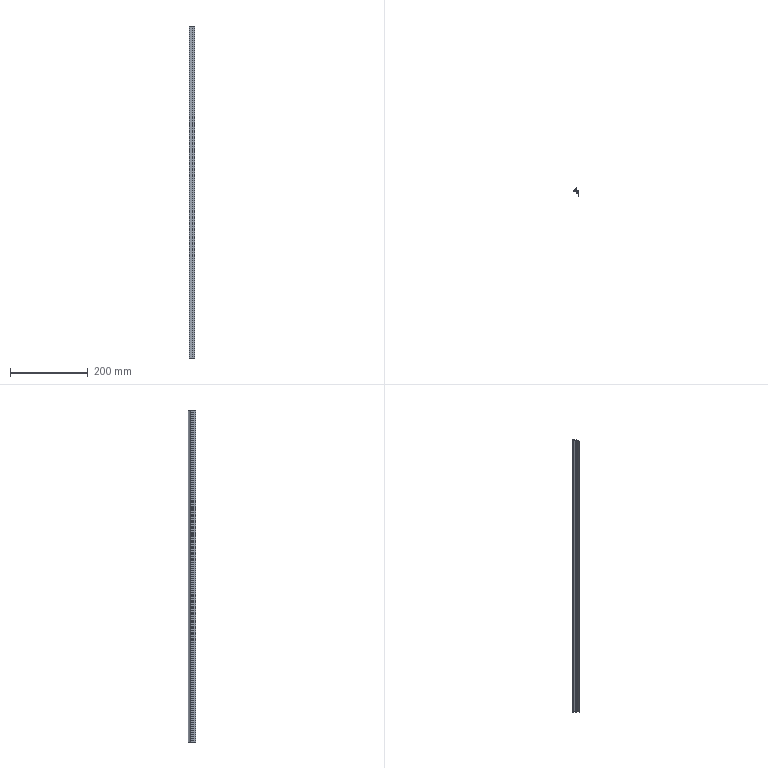Part | SolidWorks | features BaseBody 1, ICE 1, MoveFace 1 | 1 solid | 27 faces | box 14 x 20.3 x 856 mm | volume 43584 mm3 | plane 20 | cylinder 7 | commonest cylinder face diameters 0.387 x2 0.8 x2 0.4 x1 20 x1 22 x1
STEP:
#1=CARTESIAN_POINT('',(-5.304,-0.625,200.));
#2=VERTEX_POINT('',#1);
#3=CARTESIAN_POINT('',(-5.449,-0.8125,200.));
#4=VERTEX_POINT('',#3);
#5=CARTESIAN_POINT('',(-5.255,-0.8125,200.));
#6=DIRECTION('',(0.,0.,1.));
#7=DIRECTION('',(-1.,0.,0.));
#8=AXIS2_PLACEMENT_3D('',#5,#6,#7);
#9=CIRCLE('',#8,0.1937);
#10=EDGE_CURVE('',#2,#4,#9,.T.);
#11=ORIENTED_EDGE('',*,*,#10,.T.);
#12=CARTESIAN_POINT('',(-5.449,-0.8125,-656.));
#13=VERTEX_POINT('',#12);
#14=CARTESIAN_POINT('',(-5.449,-0.8125,230.));
#15=DIRECTION('',(0.,0.,-1.));
#16=VECTOR('',#15,1000.);
#17=LINE('',#14,#16);
#18=EDGE_CURVE('',#4,#13,#17,.T.);
#19=ORIENTED_EDGE('',*,*,#18,.T.);
#20=CARTESIAN_POINT('',(-5.304,-0.625,-656.));
#21=VERTEX_POINT('',#20);
#22=CARTESIAN_POINT('',(-5.255,-0.8125,-656.));
#23=DIRECTION('',(0.,0.,-1.));
#24=DIRECTION('',(1.,0.,0.));
#25=AXIS2_PLACEMENT_3D('',#22,#23,#24);
#26=CIRCLE('',#25,0.1937);
#27=EDGE_CURVE('',#13,#21,#26,.T.);
#28=ORIENTED_EDGE('',*,*,#27,.T.);
#29=CARTESIAN_POINT('',(-5.304,-0.625,230.));
#30=DIRECTION('',(0.,0.,-1.));
#31=VECTOR('',#30,1000.);
#32=LINE('',#29,#31);
#33=EDGE_CURVE('',#2,#21,#32,.T.);
#34=ORIENTED_EDGE('',*,*,#33,.F.);
#35=EDGE_LOOP('',(#11,#19,#28,#34));
#36=FACE_OUTER_BOUND('',#35,.T.);
#37=CARTESIAN_POINT('',(-5.255,-0.8125,230.));
#38=DIRECTION('',(0.,0.,-1.));
#39=DIRECTION('',(-1.,0.,0.));
#40=AXIS2_PLACEMENT_3D('',#37,#38,#39);
#41=CYLINDRICAL_SURFACE('',#40,0.1937);
#42=ADVANCED_FACE('',(#36),#41,.F.);
#43=CARTESIAN_POINT('',(5.,-1.,-656.));
#44=VERTEX_POINT('',#43);
#45=CARTESIAN_POINT('',(5.,-14.3,-656.));
#46=VERTEX_POINT('',#45);
#47=CARTESIAN_POINT('',(5.,29.623,-656.));
#48=DIRECTION('',(0.,-1.,0.));
#49=VECTOR('',#48,1000.);
#50=LINE('',#47,#49);
#51=EDGE_CURVE('',#44,#46,#50,.T.);
#52=ORIENTED_EDGE('',*,*,#51,.F.);
#53=CARTESIAN_POINT('',(5.,-1.,200.));
#54=VERTEX_POINT('',#53);
#55=CARTESIAN_POINT('',(5.,-1.,230.));
#56=DIRECTION('',(0.,0.,-1.));
#57=VECTOR('',#56,1000.);
#58=LINE('',#55,#57);
#59=EDGE_CURVE('',#54,#44,#58,.T.);
#60=ORIENTED_EDGE('',*,*,#59,.F.);
#61=CARTESIAN_POINT('',(5.,-14.3,200.));
#62=VERTEX_POINT('',#61);
#63=CARTESIAN_POINT('',(5.,-14.3,200.));
#64=DIRECTION('',(0.,1.,0.));
#65=VECTOR('',#64,1000.);
#66=LINE('',#63,#65);
#67=EDGE_CURVE('',#62,#54,#66,.T.);
#68=ORIENTED_EDGE('',*,*,#67,.F.);
#69=CARTESIAN_POINT('',(5.,-14.3,230.));
#70=DIRECTION('',(0.,0.,1.));
#71=VECTOR('',#70,1000.);
#72=LINE('',#69,#71);
#73=EDGE_CURVE('',#46,#62,#72,.T.);
#74=ORIENTED_EDGE('',*,*,#73,.F.);
#75=EDGE_LOOP('',(#52,#60,#68,#74));
#76=FACE_OUTER_BOUND('',#75,.T.);
#77=CARTESIAN_POINT('',(5.,-14.3,230.));
#78=DIRECTION('',(-1.,0.,0.));
#79=DIRECTION('',(0.,0.,1.));
#80=AXIS2_PLACEMENT_3D('',#77,#78,#79);
#81=PLANE('',#80);
#82=ADVANCED_FACE('',(#76),#81,.F.);
#83=CARTESIAN_POINT('',(-9.,-2.,-656.));
#84=VERTEX_POINT('',#83);
#85=CARTESIAN_POINT('',(-9.,-2.,200.));
#86=VERTEX_POINT('',#85);
#87=CARTESIAN_POINT('',(-9.,-2.,230.));
#88=DIRECTION('',(0.,0.,1.));
#89=VECTOR('',#88,1000.);
#90=LINE('',#87,#89);
#91=EDGE_CURVE('',#84,#86,#90,.T.);
#92=ORIENTED_EDGE('',*,*,#91,.F.);
#93=CARTESIAN_POINT('',(0.9,-2.,-656.));
#94=VERTEX_POINT('',#93);
#95=CARTESIAN_POINT('',(5.,-2.,-656.));
#96=DIRECTION('',(-1.,0.,0.));
#97=VECTOR('',#96,1000.);
#98=LINE('',#95,#97);
#99=EDGE_CURVE('',#94,#84,#98,.T.);
#100=ORIENTED_EDGE('',*,*,#99,.F.);
#101=CARTESIAN_POINT('',(0.9,-2.,200.));
#102=VERTEX_POINT('',#101);
#103=CARTESIAN_POINT('',(0.9,-2.,230.));
#104=DIRECTION('',(0.,0.,-1.));
#105=VECTOR('',#104,1000.);
#106=LINE('',#103,#105);
#107=EDGE_CURVE('',#102,#94,#106,.T.);
#108=ORIENTED_EDGE('',*,*,#107,.F.);
#109=CARTESIAN_POINT('',(5.,-2.,200.));
#110=DIRECTION('',(1.,0.,0.));
#111=VECTOR('',#110,1000.);
#112=LINE('',#109,#111);
#113=EDGE_CURVE('',#86,#102,#112,.T.);
#114=ORIENTED_EDGE('',*,*,#113,.F.);
#115=EDGE_LOOP('',(#92,#100,#108,#114));
#116=FACE_OUTER_BOUND('',#115,.T.);
#117=CARTESIAN_POINT('',(-9.,-2.,230.));
#118=DIRECTION('',(0.,1.,0.));
#119=DIRECTION('',(0.,0.,1.));
#120=AXIS2_PLACEMENT_3D('',#117,#118,#119);
#121=PLANE('',#120);
#122=ADVANCED_FACE('',(#116),#121,.F.);
#123=CARTESIAN_POINT('',(4.,-6.,200.));
#124=VERTEX_POINT('',#123);
#125=CARTESIAN_POINT('',(4.,-3.,200.));
#126=VERTEX_POINT('',#125);
#127=CARTESIAN_POINT('',(4.,29.623,200.));
#128=DIRECTION('',(0.,1.,0.));
#129=VECTOR('',#128,1000.);
#130=LINE('',#127,#129);
#131=EDGE_CURVE('',#124,#126,#130,.T.);
#132=ORIENTED_EDGE('',*,*,#131,.F.);
#133=CARTESIAN_POINT('',(1.,-6.,200.));
#134=VERTEX_POINT('',#133);
#135=CARTESIAN_POINT('',(5.,-6.,200.));
#136=DIRECTION('',(1.,0.,0.));
#137=VECTOR('',#136,1000.);
#138=LINE('',#135,#137);
#139=EDGE_CURVE('',#134,#124,#138,.T.);
#140=ORIENTED_EDGE('',*,*,#139,.F.);
#141=CARTESIAN_POINT('',(1.,-6.7,200.));
#142=VERTEX_POINT('',#141);
#143=CARTESIAN_POINT('',(1.,-6.,200.));
#144=DIRECTION('',(0.,-1.,0.));
#145=VECTOR('',#144,1000.);
#146=LINE('',#143,#145);
#147=EDGE_CURVE('',#134,#142,#146,.T.);
#148=ORIENTED_EDGE('',*,*,#147,.T.);
#149=CARTESIAN_POINT('',(-1.7,-6.7,200.));
#150=VERTEX_POINT('',#149);
#151=CARTESIAN_POINT('',(5.,-6.7,200.));
#152=DIRECTION('',(1.,0.,0.));
#153=VECTOR('',#152,1000.);
#154=LINE('',#151,#153);
#155=EDGE_CURVE('',#150,#142,#154,.T.);
#156=ORIENTED_EDGE('',*,*,#155,.F.);
#157=CARTESIAN_POINT('',(-1.7,-7.7,200.));
#158=VERTEX_POINT('',#157);
#159=CARTESIAN_POINT('',(-1.7,-6.7,200.));
#160=DIRECTION('',(0.,-1.,0.));
#161=VECTOR('',#160,1000.);
#162=LINE('',#159,#161);
#163=EDGE_CURVE('',#150,#158,#162,.T.);
#164=ORIENTED_EDGE('',*,*,#163,.T.);
#165=CARTESIAN_POINT('',(4.,-7.7,200.));
#166=VERTEX_POINT('',#165);
#167=CARTESIAN_POINT('',(5.,-7.7,200.));
#168=DIRECTION('',(-1.,0.,0.));
#169=VECTOR('',#168,1000.);
#170=LINE('',#167,#169);
#171=EDGE_CURVE('',#166,#158,#170,.T.);
#172=ORIENTED_EDGE('',*,*,#171,.F.);
#173=CARTESIAN_POINT('',(4.,-14.3,200.));
#174=VERTEX_POINT('',#173);
#175=CARTESIAN_POINT('',(4.,29.623,200.));
#176=DIRECTION('',(0.,1.,0.));
#177=VECTOR('',#176,1000.);
#178=LINE('',#175,#177);
#179=EDGE_CURVE('',#174,#166,#178,.T.);
#180=ORIENTED_EDGE('',*,*,#179,.F.);
#181=CARTESIAN_POINT('',(5.,-14.3,200.));
#182=DIRECTION('',(-1.,0.,0.));
#183=VECTOR('',#182,1000.);
#184=LINE('',#181,#183);
#185=EDGE_CURVE('',#62,#174,#184,.T.);
#186=ORIENTED_EDGE('',*,*,#185,.F.);
#187=ORIENTED_EDGE('',*,*,#67,.T.);
#188=CARTESIAN_POINT('',(-5.207,-1.,200.));
#189=VERTEX_POINT('',#188);
#190=CARTESIAN_POINT('',(5.,-1.,200.));
#191=DIRECTION('',(1.,0.,0.));
#192=VECTOR('',#191,1000.);
#193=LINE('',#190,#192);
#194=EDGE_CURVE('',#189,#54,#193,.T.);
#195=ORIENTED_EDGE('',*,*,#194,.F.);
#196=CARTESIAN_POINT('',(-5.255,-0.8125,200.));
#197=DIRECTION('',(0.,0.,1.));
#198=DIRECTION('',(-1.,0.,0.));
#199=AXIS2_PLACEMENT_3D('',#196,#197,#198);
#200=CIRCLE('',#199,0.1937);
#201=EDGE_CURVE('',#4,#189,#200,.T.);
#202=ORIENTED_EDGE('',*,*,#201,.F.);
#203=ORIENTED_EDGE('',*,*,#10,.F.);
#204=CARTESIAN_POINT('',(-1.368,3.063,200.));
#205=VERTEX_POINT('',#204);
#206=CARTESIAN_POINT('',(-10.628,9.,200.));
#207=DIRECTION('',(0.,0.,1.));
#208=DIRECTION('',(-1.,0.,0.));
#209=AXIS2_PLACEMENT_3D('',#206,#207,#208);
#210=CIRCLE('',#209,11.);
#211=EDGE_CURVE('',#2,#205,#210,.T.);
#212=ORIENTED_EDGE('',*,*,#211,.T.);
#213=CARTESIAN_POINT('',(-1.,2.955,200.));
#214=VERTEX_POINT('',#213);
#215=CARTESIAN_POINT('',(-1.2,2.955,200.));
#216=DIRECTION('',(0.,0.,1.));
#217=DIRECTION('',(-1.,0.,0.));
#218=AXIS2_PLACEMENT_3D('',#215,#216,#217);
#219=CIRCLE('',#218,0.2);
#220=EDGE_CURVE('',#214,#205,#219,.T.);
#221=ORIENTED_EDGE('',*,*,#220,.F.);
#222=CARTESIAN_POINT('',(-1.,1.5,200.));
#223=VERTEX_POINT('',#222);
#224=CARTESIAN_POINT('',(-1.,2.955,200.));
#225=DIRECTION('',(0.,1.,0.));
#226=VECTOR('',#225,1000.);
#227=LINE('',#224,#226);
#228=EDGE_CURVE('',#223,#214,#227,.T.);
#229=ORIENTED_EDGE('',*,*,#228,.F.);
#230=CARTESIAN_POINT('',(0.,1.5,200.));
#231=VERTEX_POINT('',#230);
#232=CARTESIAN_POINT('',(-1.,1.5,200.));
#233=DIRECTION('',(-1.,0.,0.));
#234=VECTOR('',#233,1000.);
#235=LINE('',#232,#234);
#236=EDGE_CURVE('',#231,#223,#235,.T.);
#237=ORIENTED_EDGE('',*,*,#236,.F.);
#238=CARTESIAN_POINT('',(0.,6.,200.));
#239=VERTEX_POINT('',#238);
#240=CARTESIAN_POINT('',(0.,1.5,200.));
#241=DIRECTION('',(0.,-1.,0.));
#242=VECTOR('',#241,1000.);
#243=LINE('',#240,#242);
#244=EDGE_CURVE('',#239,#231,#243,.T.);
#245=ORIENTED_EDGE('',*,*,#244,.F.);
#246=CARTESIAN_POINT('',(-0.8,6.,200.));
#247=VERTEX_POINT('',#246);
#248=CARTESIAN_POINT('',(0.,6.,200.));
#249=DIRECTION('',(1.,0.,0.));
#250=VECTOR('',#249,1000.);
#251=LINE('',#248,#250);
#252=EDGE_CURVE('',#247,#239,#251,.T.);
#253=ORIENTED_EDGE('',*,*,#252,.F.);
#254=CARTESIAN_POINT('',(-1.178,5.731,200.));
#255=VERTEX_POINT('',#254);
#256=CARTESIAN_POINT('',(-0.8,5.6,200.));
#257=DIRECTION('',(0.,0.,1.));
#258=DIRECTION('',(-1.,0.,0.));
#259=AXIS2_PLACEMENT_3D('',#256,#257,#258);
#260=CIRCLE('',#259,0.4);
#261=EDGE_CURVE('',#247,#255,#260,.T.);
#262=ORIENTED_EDGE('',*,*,#261,.T.);
#263=CARTESIAN_POINT('',(-8.678,-0.8077,200.));
#264=VERTEX_POINT('',#263);
#265=CARTESIAN_POINT('',(-10.628,9.,200.));
#266=DIRECTION('',(0.,0.,1.));
#267=DIRECTION('',(-1.,0.,0.));
#268=AXIS2_PLACEMENT_3D('',#265,#266,#267);
#269=CIRCLE('',#268,10.);
#270=EDGE_CURVE('',#264,#255,#269,.T.);
#271=ORIENTED_EDGE('',*,*,#270,.F.);
#272=CARTESIAN_POINT('',(-9.,-1.2,200.));
#273=VERTEX_POINT('',#272);
#274=CARTESIAN_POINT('',(-8.6,-1.2,200.));
#275=DIRECTION('',(0.,0.,1.));
#276=DIRECTION('',(-1.,0.,0.));
#277=AXIS2_PLACEMENT_3D('',#274,#275,#276);
#278=CIRCLE('',#277,0.4);
#279=EDGE_CURVE('',#264,#273,#278,.T.);
#280=ORIENTED_EDGE('',*,*,#279,.T.);
#281=CARTESIAN_POINT('',(-9.,8.,200.));
#282=DIRECTION('',(0.,-1.,0.));
#283=VECTOR('',#282,1000.);
#284=LINE('',#281,#283);
#285=EDGE_CURVE('',#273,#86,#284,.T.);
#286=ORIENTED_EDGE('',*,*,#285,.T.);
#287=ORIENTED_EDGE('',*,*,#113,.T.);
#288=CARTESIAN_POINT('',(0.9,-3.,200.));
#289=VERTEX_POINT('',#288);
#290=CARTESIAN_POINT('',(0.9,29.623,200.));
#291=DIRECTION('',(0.,1.,0.));
#292=VECTOR('',#291,1000.);
#293=LINE('',#290,#292);
#294=EDGE_CURVE('',#289,#102,#293,.T.);
#295=ORIENTED_EDGE('',*,*,#294,.F.);
#296=CARTESIAN_POINT('',(5.,-3.,200.));
#297=DIRECTION('',(-1.,0.,0.));
#298=VECTOR('',#297,1000.);
#299=LINE('',#296,#298);
#300=EDGE_CURVE('',#126,#289,#299,.T.);
#301=ORIENTED_EDGE('',*,*,#300,.F.);
#302=EDGE_LOOP('',(#132,#140,#148,#156,#164,#172,#180,#186,#187,#195,#202,#203,#212,#221,#229,#237,#245,#253,#262,#271,#280,#286,#287,#295,#301));
#303=FACE_OUTER_BOUND('',#302,.T.);
#304=CARTESIAN_POINT('',(5.,29.623,200.));
#305=DIRECTION('',(0.,0.,-1.));
#306=DIRECTION('',(-1.,0.,0.));
#307=AXIS2_PLACEMENT_3D('',#304,#305,#306);
#308=PLANE('',#307);
#309=ADVANCED_FACE('',(#303),#308,.F.);
#310=ORIENTED_EDGE('',*,*,#185,.T.);
#311=CARTESIAN_POINT('',(4.,-14.3,-656.));
#312=VERTEX_POINT('',#311);
#313=CARTESIAN_POINT('',(4.,-14.3,230.));
#314=DIRECTION('',(0.,0.,1.));
#315=VECTOR('',#314,1000.);
#316=LINE('',#313,#315);
#317=EDGE_CURVE('',#312,#174,#316,.T.);
#318=ORIENTED_EDGE('',*,*,#317,.F.);
#319=CARTESIAN_POINT('',(5.,-14.3,-656.));
#320=DIRECTION('',(-1.,0.,0.));
#321=VECTOR('',#320,1000.);
#322=LINE('',#319,#321);
#323=EDGE_CURVE('',#46,#312,#322,.T.);
#324=ORIENTED_EDGE('',*,*,#323,.F.);
#325=ORIENTED_EDGE('',*,*,#73,.T.);
#326=EDGE_LOOP('',(#310,#318,#324,#325));
#327=FACE_OUTER_BOUND('',#326,.T.);
#328=CARTESIAN_POINT('',(4.,-14.3,230.));
#329=DIRECTION('',(0.,1.,0.));
#330=DIRECTION('',(0.,0.,1.));
#331=AXIS2_PLACEMENT_3D('',#328,#329,#330);
#332=PLANE('',#331);
#333=ADVANCED_FACE('',(#327),#332,.F.);
#334=ORIENTED_EDGE('',*,*,#51,.T.);
#335=ORIENTED_EDGE('',*,*,#323,.T.);
#336=CARTESIAN_POINT('',(4.,-7.7,-656.));
#337=VERTEX_POINT('',#336);
#338=CARTESIAN_POINT('',(4.,-7.7,-656.));
#339=DIRECTION('',(0.,-1.,0.));
#340=VECTOR('',#339,1000.);
#341=LINE('',#338,#340);
#342=EDGE_CURVE('',#337,#312,#341,.T.);
#343=ORIENTED_EDGE('',*,*,#342,.F.);
#344=CARTESIAN_POINT('',(-1.7,-7.7,-656.));
#345=VERTEX_POINT('',#344);
#346=CARTESIAN_POINT('',(-1.7,-7.7,-656.));
#347=DIRECTION('',(1.,0.,0.));
#348=VECTOR('',#347,1000.);
#349=LINE('',#346,#348);
#350=EDGE_CURVE('',#345,#337,#349,.T.);
#351=ORIENTED_EDGE('',*,*,#350,.F.);
#352=CARTESIAN_POINT('',(-1.7,-6.7,-656.));
#353=VERTEX_POINT('',#352);
#354=CARTESIAN_POINT('',(-1.7,29.623,-656.));
#355=DIRECTION('',(0.,1.,0.));
#356=VECTOR('',#355,1000.);
#357=LINE('',#354,#356);
#358=EDGE_CURVE('',#345,#353,#357,.T.);
#359=ORIENTED_EDGE('',*,*,#358,.T.);
#360=CARTESIAN_POINT('',(1.,-6.7,-656.));
#361=VERTEX_POINT('',#360);
#362=CARTESIAN_POINT('',(1.,-6.7,-656.));
#363=DIRECTION('',(-1.,0.,0.));
#364=VECTOR('',#363,1000.);
#365=LINE('',#362,#364);
#366=EDGE_CURVE('',#361,#353,#365,.T.);
#367=ORIENTED_EDGE('',*,*,#366,.F.);
#368=CARTESIAN_POINT('',(1.,-6.,-656.));
#369=VERTEX_POINT('',#368);
#370=CARTESIAN_POINT('',(1.,29.623,-656.));
#371=DIRECTION('',(0.,1.,0.));
#372=VECTOR('',#371,1000.);
#373=LINE('',#370,#372);
#374=EDGE_CURVE('',#361,#369,#373,.T.);
#375=ORIENTED_EDGE('',*,*,#374,.T.);
#376=CARTESIAN_POINT('',(4.,-6.,-656.));
#377=VERTEX_POINT('',#376);
#378=CARTESIAN_POINT('',(4.,-6.,-656.));
#379=DIRECTION('',(-1.,0.,0.));
#380=VECTOR('',#379,1000.);
#381=LINE('',#378,#380);
#382=EDGE_CURVE('',#377,#369,#381,.T.);
#383=ORIENTED_EDGE('',*,*,#382,.F.);
#384=CARTESIAN_POINT('',(4.,-3.,-656.));
#385=VERTEX_POINT('',#384);
#386=CARTESIAN_POINT('',(4.,-3.,-656.));
#387=DIRECTION('',(0.,-1.,0.));
#388=VECTOR('',#387,1000.);
#389=LINE('',#386,#388);
#390=EDGE_CURVE('',#385,#377,#389,.T.);
#391=ORIENTED_EDGE('',*,*,#390,.F.);
#392=CARTESIAN_POINT('',(0.9,-3.,-656.));
#393=VERTEX_POINT('',#392);
#394=CARTESIAN_POINT('',(0.9,-3.,-656.));
#395=DIRECTION('',(1.,0.,0.));
#396=VECTOR('',#395,1000.);
#397=LINE('',#394,#396);
#398=EDGE_CURVE('',#393,#385,#397,.T.);
#399=ORIENTED_EDGE('',*,*,#398,.F.);
#400=CARTESIAN_POINT('',(0.9,-2.,-656.));
#401=DIRECTION('',(0.,-1.,0.));
#402=VECTOR('',#401,1000.);
#403=LINE('',#400,#402);
#404=EDGE_CURVE('',#94,#393,#403,.T.);
#405=ORIENTED_EDGE('',*,*,#404,.F.);
#406=ORIENTED_EDGE('',*,*,#99,.T.);
#407=CARTESIAN_POINT('',(-9.,-1.2,-656.));
#408=VERTEX_POINT('',#407);
#409=CARTESIAN_POINT('',(-9.,-1.2,-656.));
#410=DIRECTION('',(0.,-1.,0.));
#411=VECTOR('',#410,1000.);
#412=LINE('',#409,#411);
#413=EDGE_CURVE('',#408,#84,#412,.T.);
#414=ORIENTED_EDGE('',*,*,#413,.F.);
#415=CARTESIAN_POINT('',(-8.678,-0.8077,-656.));
#416=VERTEX_POINT('',#415);
#417=CARTESIAN_POINT('',(-8.6,-1.2,-656.));
#418=DIRECTION('',(0.,0.,-1.));
#419=DIRECTION('',(1.,0.,0.));
#420=AXIS2_PLACEMENT_3D('',#417,#418,#419);
#421=CIRCLE('',#420,0.4);
#422=EDGE_CURVE('',#408,#416,#421,.T.);
#423=ORIENTED_EDGE('',*,*,#422,.T.);
#424=CARTESIAN_POINT('',(-1.178,5.731,-656.));
#425=VERTEX_POINT('',#424);
#426=CARTESIAN_POINT('',(-10.628,9.,-656.));
#427=DIRECTION('',(0.,0.,-1.));
#428=DIRECTION('',(1.,0.,0.));
#429=AXIS2_PLACEMENT_3D('',#426,#427,#428);
#430=CIRCLE('',#429,10.);
#431=EDGE_CURVE('',#425,#416,#430,.T.);
#432=ORIENTED_EDGE('',*,*,#431,.F.);
#433=CARTESIAN_POINT('',(-0.8,6.,-656.));
#434=VERTEX_POINT('',#433);
#435=CARTESIAN_POINT('',(-0.8,5.6,-656.));
#436=DIRECTION('',(0.,0.,-1.));
#437=DIRECTION('',(1.,0.,0.));
#438=AXIS2_PLACEMENT_3D('',#435,#436,#437);
#439=CIRCLE('',#438,0.4);
#440=EDGE_CURVE('',#425,#434,#439,.T.);
#441=ORIENTED_EDGE('',*,*,#440,.T.);
#442=CARTESIAN_POINT('',(0.,6.,-656.));
#443=VERTEX_POINT('',#442);
#444=CARTESIAN_POINT('',(0.,6.,-656.));
#445=DIRECTION('',(-1.,0.,0.));
#446=VECTOR('',#445,1000.);
#447=LINE('',#444,#446);
#448=EDGE_CURVE('',#443,#434,#447,.T.);
#449=ORIENTED_EDGE('',*,*,#448,.F.);
#450=CARTESIAN_POINT('',(0.,1.5,-656.));
#451=VERTEX_POINT('',#450);
#452=CARTESIAN_POINT('',(0.,1.5,-656.));
#453=DIRECTION('',(0.,1.,0.));
#454=VECTOR('',#453,1000.);
#455=LINE('',#452,#454);
#456=EDGE_CURVE('',#451,#443,#455,.T.);
#457=ORIENTED_EDGE('',*,*,#456,.F.);
#458=CARTESIAN_POINT('',(-1.,1.5,-656.));
#459=VERTEX_POINT('',#458);
#460=CARTESIAN_POINT('',(-1.,1.5,-656.));
#461=DIRECTION('',(1.,0.,0.));
#462=VECTOR('',#461,1000.);
#463=LINE('',#460,#462);
#464=EDGE_CURVE('',#459,#451,#463,.T.);
#465=ORIENTED_EDGE('',*,*,#464,.F.);
#466=CARTESIAN_POINT('',(-1.,2.955,-656.));
#467=VERTEX_POINT('',#466);
#468=CARTESIAN_POINT('',(-1.,2.955,-656.));
#469=DIRECTION('',(0.,-1.,0.));
#470=VECTOR('',#469,1000.);
#471=LINE('',#468,#470);
#472=EDGE_CURVE('',#467,#459,#471,.T.);
#473=ORIENTED_EDGE('',*,*,#472,.F.);
#474=CARTESIAN_POINT('',(-1.368,3.063,-656.));
#475=VERTEX_POINT('',#474);
#476=CARTESIAN_POINT('',(-1.2,2.955,-656.));
#477=DIRECTION('',(0.,0.,-1.));
#478=DIRECTION('',(1.,0.,0.));
#479=AXIS2_PLACEMENT_3D('',#476,#477,#478);
#480=CIRCLE('',#479,0.2);
#481=EDGE_CURVE('',#475,#467,#480,.T.);
#482=ORIENTED_EDGE('',*,*,#481,.F.);
#483=CARTESIAN_POINT('',(-10.628,9.,-656.));
#484=DIRECTION('',(0.,0.,-1.));
#485=DIRECTION('',(1.,0.,0.));
#486=AXIS2_PLACEMENT_3D('',#483,#484,#485);
#487=CIRCLE('',#486,11.);
#488=EDGE_CURVE('',#475,#21,#487,.T.);
#489=ORIENTED_EDGE('',*,*,#488,.T.);
#490=ORIENTED_EDGE('',*,*,#27,.F.);
#491=CARTESIAN_POINT('',(-5.207,-1.,-656.));
#492=VERTEX_POINT('',#491);
#493=CARTESIAN_POINT('',(-5.255,-0.8125,-656.));
#494=DIRECTION('',(0.,0.,-1.));
#495=DIRECTION('',(1.,0.,0.));
#496=AXIS2_PLACEMENT_3D('',#493,#494,#495);
#497=CIRCLE('',#496,0.1937);
#498=EDGE_CURVE('',#492,#13,#497,.T.);
#499=ORIENTED_EDGE('',*,*,#498,.F.);
#500=CARTESIAN_POINT('',(5.,-1.,-656.));
#501=DIRECTION('',(-1.,0.,0.));
#502=VECTOR('',#501,1000.);
#503=LINE('',#500,#502);
#504=EDGE_CURVE('',#44,#492,#503,.T.);
#505=ORIENTED_EDGE('',*,*,#504,.F.);
#506=EDGE_LOOP('',(#334,#335,#343,#351,#359,#367,#375,#383,#391,#399,#405,#406,#414,#423,#432,#441,#449,#457,#465,#473,#482,#489,#490,#499,#505));
#507=FACE_OUTER_BOUND('',#506,.T.);
#508=CARTESIAN_POINT('',(5.,29.623,-656.));
#509=DIRECTION('',(0.,0.,1.));
#510=DIRECTION('',(1.,0.,0.));
#511=AXIS2_PLACEMENT_3D('',#508,#509,#510);
#512=PLANE('',#511);
#513=ADVANCED_FACE('',(#507),#512,.F.);
#514=ORIENTED_EDGE('',*,*,#59,.T.);
#515=ORIENTED_EDGE('',*,*,#504,.T.);
#516=CARTESIAN_POINT('',(-5.207,-1.,230.));
#517=DIRECTION('',(0.,0.,-1.));
#518=VECTOR('',#517,1000.);
#519=LINE('',#516,#518);
#520=EDGE_CURVE('',#189,#492,#519,.T.);
#521=ORIENTED_EDGE('',*,*,#520,.F.);
#522=ORIENTED_EDGE('',*,*,#194,.T.);
#523=EDGE_LOOP('',(#514,#515,#521,#522));
#524=FACE_OUTER_BOUND('',#523,.T.);
#525=CARTESIAN_POINT('',(5.,-1.,230.));
#526=DIRECTION('',(0.,-1.,0.));
#527=DIRECTION('',(0.,0.,-1.));
#528=AXIS2_PLACEMENT_3D('',#525,#526,#527);
#529=PLANE('',#528);
#530=ADVANCED_FACE('',(#524),#529,.F.);
#531=CARTESIAN_POINT('',(-9.,-1.2,230.));
#532=DIRECTION('',(0.,0.,1.));
#533=VECTOR('',#532,1000.);
#534=LINE('',#531,#533);
#535=EDGE_CURVE('',#408,#273,#534,.T.);
#536=ORIENTED_EDGE('',*,*,#535,.F.);
#537=ORIENTED_EDGE('',*,*,#413,.T.);
#538=ORIENTED_EDGE('',*,*,#91,.T.);
#539=ORIENTED_EDGE('',*,*,#285,.F.);
#540=EDGE_LOOP('',(#536,#537,#538,#539));
#541=FACE_OUTER_BOUND('',#540,.T.);
#542=CARTESIAN_POINT('',(-9.,-1.2,230.));
#543=DIRECTION('',(1.,0.,0.));
#544=DIRECTION('',(0.,0.,-1.));
#545=AXIS2_PLACEMENT_3D('',#542,#543,#544);
#546=PLANE('',#545);
#547=ADVANCED_FACE('',(#541),#546,.F.);
#548=ORIENTED_EDGE('',*,*,#294,.T.);
#549=ORIENTED_EDGE('',*,*,#107,.T.);
#550=ORIENTED_EDGE('',*,*,#404,.T.);
#551=CARTESIAN_POINT('',(0.9,-3.,230.));
#552=DIRECTION('',(0.,0.,-1.));
#553=VECTOR('',#552,1000.);
#554=LINE('',#551,#553);
#555=EDGE_CURVE('',#289,#393,#554,.T.);
#556=ORIENTED_EDGE('',*,*,#555,.F.);
#557=EDGE_LOOP('',(#548,#549,#550,#556));
#558=FACE_OUTER_BOUND('',#557,.T.);
#559=CARTESIAN_POINT('',(0.9,-2.,230.));
#560=DIRECTION('',(1.,0.,0.));
#561=DIRECTION('',(0.,0.,-1.));
#562=AXIS2_PLACEMENT_3D('',#559,#560,#561);
#563=PLANE('',#562);
#564=ADVANCED_FACE('',(#558),#563,.F.);
#565=ORIENTED_EDGE('',*,*,#300,.T.);
#566=ORIENTED_EDGE('',*,*,#555,.T.);
#567=ORIENTED_EDGE('',*,*,#398,.T.);
#568=CARTESIAN_POINT('',(4.,-3.,230.));
#569=DIRECTION('',(0.,0.,-1.));
#570=VECTOR('',#569,1000.);
#571=LINE('',#568,#570);
#572=EDGE_CURVE('',#126,#385,#571,.T.);
#573=ORIENTED_EDGE('',*,*,#572,.F.);
#574=EDGE_LOOP('',(#565,#566,#567,#573));
#575=FACE_OUTER_BOUND('',#574,.T.);
#576=CARTESIAN_POINT('',(0.9,-3.,230.));
#577=DIRECTION('',(0.,1.,0.));
#578=DIRECTION('',(0.,0.,1.));
#579=AXIS2_PLACEMENT_3D('',#576,#577,#578);
#580=PLANE('',#579);
#581=ADVANCED_FACE('',(#575),#580,.F.);
#582=ORIENTED_EDGE('',*,*,#131,.T.);
#583=ORIENTED_EDGE('',*,*,#572,.T.);
#584=ORIENTED_EDGE('',*,*,#390,.T.);
#585=CARTESIAN_POINT('',(4.,-6.,230.));
#586=DIRECTION('',(0.,0.,-1.));
#587=VECTOR('',#586,1000.);
#588=LINE('',#585,#587);
#589=EDGE_CURVE('',#124,#377,#588,.T.);
#590=ORIENTED_EDGE('',*,*,#589,.F.);
#591=EDGE_LOOP('',(#582,#583,#584,#590));
#592=FACE_OUTER_BOUND('',#591,.T.);
#593=CARTESIAN_POINT('',(4.,-3.,230.));
#594=DIRECTION('',(1.,0.,0.));
#595=DIRECTION('',(0.,0.,-1.));
#596=AXIS2_PLACEMENT_3D('',#593,#594,#595);
#597=PLANE('',#596);
#598=ADVANCED_FACE('',(#592),#597,.F.);
#599=ORIENTED_EDGE('',*,*,#139,.T.);
#600=ORIENTED_EDGE('',*,*,#589,.T.);
#601=ORIENTED_EDGE('',*,*,#382,.T.);
#602=CARTESIAN_POINT('',(1.,-6.,230.));
#603=DIRECTION('',(0.,0.,-1.));
#604=VECTOR('',#603,1000.);
#605=LINE('',#602,#604);
#606=EDGE_CURVE('',#134,#369,#605,.T.);
#607=ORIENTED_EDGE('',*,*,#606,.F.);
#608=EDGE_LOOP('',(#599,#600,#601,#607));
#609=FACE_OUTER_BOUND('',#608,.T.);
#610=CARTESIAN_POINT('',(4.,-6.,230.));
#611=DIRECTION('',(0.,-1.,0.));
#612=DIRECTION('',(0.,0.,-1.));
#613=AXIS2_PLACEMENT_3D('',#610,#611,#612);
#614=PLANE('',#613);
#615=ADVANCED_FACE('',(#609),#614,.F.);
#616=ORIENTED_EDGE('',*,*,#155,.T.);
#617=CARTESIAN_POINT('',(1.,-6.7,230.));
#618=DIRECTION('',(0.,0.,1.));
#619=VECTOR('',#618,1000.);
#620=LINE('',#617,#619);
#621=EDGE_CURVE('',#361,#142,#620,.T.);
#622=ORIENTED_EDGE('',*,*,#621,.F.);
#623=ORIENTED_EDGE('',*,*,#366,.T.);
#624=CARTESIAN_POINT('',(-1.7,-6.7,230.));
#625=DIRECTION('',(0.,0.,-1.));
#626=VECTOR('',#625,1000.);
#627=LINE('',#624,#626);
#628=EDGE_CURVE('',#150,#353,#627,.T.);
#629=ORIENTED_EDGE('',*,*,#628,.F.);
#630=EDGE_LOOP('',(#616,#622,#623,#629));
#631=FACE_OUTER_BOUND('',#630,.T.);
#632=CARTESIAN_POINT('',(1.,-6.7,230.));
#633=DIRECTION('',(0.,-1.,0.));
#634=DIRECTION('',(0.,0.,-1.));
#635=AXIS2_PLACEMENT_3D('',#632,#633,#634);
#636=PLANE('',#635);
#637=ADVANCED_FACE('',(#631),#636,.F.);
#638=ORIENTED_EDGE('',*,*,#171,.T.);
#639=CARTESIAN_POINT('',(-1.7,-7.7,230.));
#640=DIRECTION('',(0.,0.,1.));
#641=VECTOR('',#640,1000.);
#642=LINE('',#639,#641);
#643=EDGE_CURVE('',#345,#158,#642,.T.);
#644=ORIENTED_EDGE('',*,*,#643,.F.);
#645=ORIENTED_EDGE('',*,*,#350,.T.);
#646=CARTESIAN_POINT('',(4.,-7.7,230.));
#647=DIRECTION('',(0.,0.,-1.));
#648=VECTOR('',#647,1000.);
#649=LINE('',#646,#648);
#650=EDGE_CURVE('',#166,#337,#649,.T.);
#651=ORIENTED_EDGE('',*,*,#650,.F.);
#652=EDGE_LOOP('',(#638,#644,#645,#651));
#653=FACE_OUTER_BOUND('',#652,.T.);
#654=CARTESIAN_POINT('',(-1.7,-7.7,230.));
#655=DIRECTION('',(0.,1.,0.));
#656=DIRECTION('',(0.,0.,1.));
#657=AXIS2_PLACEMENT_3D('',#654,#655,#656);
#658=PLANE('',#657);
#659=ADVANCED_FACE('',(#653),#658,.F.);
#660=ORIENTED_EDGE('',*,*,#179,.T.);
#661=ORIENTED_EDGE('',*,*,#650,.T.);
#662=ORIENTED_EDGE('',*,*,#342,.T.);
#663=ORIENTED_EDGE('',*,*,#317,.T.);
#664=EDGE_LOOP('',(#660,#661,#662,#663));
#665=FACE_OUTER_BOUND('',#664,.T.);
#666=CARTESIAN_POINT('',(4.,-7.7,230.));
#667=DIRECTION('',(1.,0.,0.));
#668=DIRECTION('',(0.,0.,-1.));
#669=AXIS2_PLACEMENT_3D('',#666,#667,#668);
#670=PLANE('',#669);
#671=ADVANCED_FACE('',(#665),#670,.F.);
#672=ORIENTED_EDGE('',*,*,#18,.F.);
#673=ORIENTED_EDGE('',*,*,#201,.T.);
#674=ORIENTED_EDGE('',*,*,#520,.T.);
#675=ORIENTED_EDGE('',*,*,#498,.T.);
#676=EDGE_LOOP('',(#672,#673,#674,#675));
#677=FACE_OUTER_BOUND('',#676,.T.);
#678=CARTESIAN_POINT('',(-5.255,-0.8125,230.));
#679=DIRECTION('',(0.,0.,-1.));
#680=DIRECTION('',(-1.,0.,0.));
#681=AXIS2_PLACEMENT_3D('',#678,#679,#680);
#682=CYLINDRICAL_SURFACE('',#681,0.1937);
#683=ADVANCED_FACE('',(#677),#682,.F.);
#684=CARTESIAN_POINT('',(-1.,2.955,230.));
#685=DIRECTION('',(0.,0.,1.));
#686=VECTOR('',#685,1000.);
#687=LINE('',#684,#686);
#688=EDGE_CURVE('',#467,#214,#687,.T.);
#689=ORIENTED_EDGE('',*,*,#688,.F.);
#690=ORIENTED_EDGE('',*,*,#472,.T.);
#691=CARTESIAN_POINT('',(-1.,1.5,230.));
#692=DIRECTION('',(0.,0.,-1.));
#693=VECTOR('',#692,1000.);
#694=LINE('',#691,#693);
#695=EDGE_CURVE('',#223,#459,#694,.T.);
#696=ORIENTED_EDGE('',*,*,#695,.F.);
#697=ORIENTED_EDGE('',*,*,#228,.T.);
#698=EDGE_LOOP('',(#689,#690,#696,#697));
#699=FACE_OUTER_BOUND('',#698,.T.);
#700=CARTESIAN_POINT('',(-1.,2.955,230.));
#701=DIRECTION('',(1.,0.,0.));
#702=DIRECTION('',(0.,0.,-1.));
#703=AXIS2_PLACEMENT_3D('',#700,#701,#702);
#704=PLANE('',#703);
#705=ADVANCED_FACE('',(#699),#704,.F.);
#706=ORIENTED_EDGE('',*,*,#488,.F.);
#707=CARTESIAN_POINT('',(-1.368,3.063,230.));
#708=DIRECTION('',(0.,0.,1.));
#709=VECTOR('',#708,1000.);
#710=LINE('',#707,#709);
#711=EDGE_CURVE('',#475,#205,#710,.T.);
#712=ORIENTED_EDGE('',*,*,#711,.T.);
#713=ORIENTED_EDGE('',*,*,#211,.F.);
#714=ORIENTED_EDGE('',*,*,#33,.T.);
#715=EDGE_LOOP('',(#706,#712,#713,#714));
#716=FACE_OUTER_BOUND('',#715,.T.);
#717=CARTESIAN_POINT('',(-10.628,9.,230.));
#718=DIRECTION('',(0.,0.,-1.));
#719=DIRECTION('',(-1.,0.,0.));
#720=AXIS2_PLACEMENT_3D('',#717,#718,#719);
#721=CYLINDRICAL_SURFACE('',#720,11.);
#722=ADVANCED_FACE('',(#716),#721,.T.);
#723=CARTESIAN_POINT('',(-1.178,5.731,230.));
#724=DIRECTION('',(0.,0.,1.));
#725=VECTOR('',#724,1000.);
#726=LINE('',#723,#725);
#727=EDGE_CURVE('',#425,#255,#726,.T.);
#728=ORIENTED_EDGE('',*,*,#727,.F.);
#729=ORIENTED_EDGE('',*,*,#431,.T.);
#730=CARTESIAN_POINT('',(-8.678,-0.8077,230.));
#731=DIRECTION('',(0.,0.,-1.));
#732=VECTOR('',#731,1000.);
#733=LINE('',#730,#732);
#734=EDGE_CURVE('',#264,#416,#733,.T.);
#735=ORIENTED_EDGE('',*,*,#734,.F.);
#736=ORIENTED_EDGE('',*,*,#270,.T.);
#737=EDGE_LOOP('',(#728,#729,#735,#736));
#738=FACE_OUTER_BOUND('',#737,.T.);
#739=CARTESIAN_POINT('',(-10.628,9.,230.));
#740=DIRECTION('',(0.,0.,-1.));
#741=DIRECTION('',(-1.,0.,0.));
#742=AXIS2_PLACEMENT_3D('',#739,#740,#741);
#743=CYLINDRICAL_SURFACE('',#742,10.);
#744=ADVANCED_FACE('',(#738),#743,.F.);
#745=CARTESIAN_POINT('',(0.,1.5,230.));
#746=DIRECTION('',(0.,0.,1.));
#747=VECTOR('',#746,1000.);
#748=LINE('',#745,#747);
#749=EDGE_CURVE('',#451,#231,#748,.T.);
#750=ORIENTED_EDGE('',*,*,#749,.F.);
#751=ORIENTED_EDGE('',*,*,#456,.T.);
#752=CARTESIAN_POINT('',(0.,6.,230.));
#753=DIRECTION('',(0.,0.,-1.));
#754=VECTOR('',#753,1000.);
#755=LINE('',#752,#754);
#756=EDGE_CURVE('',#239,#443,#755,.T.);
#757=ORIENTED_EDGE('',*,*,#756,.F.);
#758=ORIENTED_EDGE('',*,*,#244,.T.);
#759=EDGE_LOOP('',(#750,#751,#757,#758));
#760=FACE_OUTER_BOUND('',#759,.T.);
#761=CARTESIAN_POINT('',(0.,1.5,230.));
#762=DIRECTION('',(-1.,0.,0.));
#763=DIRECTION('',(0.,0.,1.));
#764=AXIS2_PLACEMENT_3D('',#761,#762,#763);
#765=PLANE('',#764);
#766=ADVANCED_FACE('',(#760),#765,.F.);
#767=ORIENTED_EDGE('',*,*,#422,.F.);
#768=ORIENTED_EDGE('',*,*,#535,.T.);
#769=ORIENTED_EDGE('',*,*,#279,.F.);
#770=ORIENTED_EDGE('',*,*,#734,.T.);
#771=EDGE_LOOP('',(#767,#768,#769,#770));
#772=FACE_OUTER_BOUND('',#771,.T.);
#773=CARTESIAN_POINT('',(-8.6,-1.2,230.));
#774=DIRECTION('',(0.,0.,-1.));
#775=DIRECTION('',(-1.,0.,0.));
#776=AXIS2_PLACEMENT_3D('',#773,#774,#775);
#777=CYLINDRICAL_SURFACE('',#776,0.4);
#778=ADVANCED_FACE('',(#772),#777,.T.);
#779=ORIENTED_EDGE('',*,*,#147,.F.);
#780=ORIENTED_EDGE('',*,*,#606,.T.);
#781=ORIENTED_EDGE('',*,*,#374,.F.);
#782=ORIENTED_EDGE('',*,*,#621,.T.);
#783=EDGE_LOOP('',(#779,#780,#781,#782));
#784=FACE_OUTER_BOUND('',#783,.T.);
#785=CARTESIAN_POINT('',(1.,-6.,230.));
#786=DIRECTION('',(1.,0.,0.));
#787=DIRECTION('',(0.,0.,-1.));
#788=AXIS2_PLACEMENT_3D('',#785,#786,#787);
#789=PLANE('',#788);
#790=ADVANCED_FACE('',(#784),#789,.F.);
#791=ORIENTED_EDGE('',*,*,#163,.F.);
#792=ORIENTED_EDGE('',*,*,#628,.T.);
#793=ORIENTED_EDGE('',*,*,#358,.F.);
#794=ORIENTED_EDGE('',*,*,#643,.T.);
#795=EDGE_LOOP('',(#791,#792,#793,#794));
#796=FACE_OUTER_BOUND('',#795,.T.);
#797=CARTESIAN_POINT('',(-1.7,-6.7,230.));
#798=DIRECTION('',(1.,0.,0.));
#799=DIRECTION('',(0.,0.,-1.));
#800=AXIS2_PLACEMENT_3D('',#797,#798,#799);
#801=PLANE('',#800);
#802=ADVANCED_FACE('',(#796),#801,.F.);
#803=ORIENTED_EDGE('',*,*,#711,.F.);
#804=ORIENTED_EDGE('',*,*,#481,.T.);
#805=ORIENTED_EDGE('',*,*,#688,.T.);
#806=ORIENTED_EDGE('',*,*,#220,.T.);
#807=EDGE_LOOP('',(#803,#804,#805,#806));
#808=FACE_OUTER_BOUND('',#807,.T.);
#809=CARTESIAN_POINT('',(-1.2,2.955,230.));
#810=DIRECTION('',(0.,0.,-1.));
#811=DIRECTION('',(-1.,0.,0.));
#812=AXIS2_PLACEMENT_3D('',#809,#810,#811);
#813=CYLINDRICAL_SURFACE('',#812,0.2);
#814=ADVANCED_FACE('',(#808),#813,.F.);
#815=ORIENTED_EDGE('',*,*,#695,.T.);
#816=ORIENTED_EDGE('',*,*,#464,.T.);
#817=ORIENTED_EDGE('',*,*,#749,.T.);
#818=ORIENTED_EDGE('',*,*,#236,.T.);
#819=EDGE_LOOP('',(#815,#816,#817,#818));
#820=FACE_OUTER_BOUND('',#819,.T.);
#821=CARTESIAN_POINT('',(-1.,1.5,230.));
#822=DIRECTION('',(0.,1.,0.));
#823=DIRECTION('',(0.,0.,1.));
#824=AXIS2_PLACEMENT_3D('',#821,#822,#823);
#825=PLANE('',#824);
#826=ADVANCED_FACE('',(#820),#825,.F.);
#827=ORIENTED_EDGE('',*,*,#440,.F.);
#828=ORIENTED_EDGE('',*,*,#727,.T.);
#829=ORIENTED_EDGE('',*,*,#261,.F.);
#830=CARTESIAN_POINT('',(-0.8,6.,230.));
#831=DIRECTION('',(0.,0.,-1.));
#832=VECTOR('',#831,1000.);
#833=LINE('',#830,#832);
#834=EDGE_CURVE('',#247,#434,#833,.T.);
#835=ORIENTED_EDGE('',*,*,#834,.T.);
#836=EDGE_LOOP('',(#827,#828,#829,#835));
#837=FACE_OUTER_BOUND('',#836,.T.);
#838=CARTESIAN_POINT('',(-0.8,5.6,230.));
#839=DIRECTION('',(0.,0.,-1.));
#840=DIRECTION('',(-1.,0.,0.));
#841=AXIS2_PLACEMENT_3D('',#838,#839,#840);
#842=CYLINDRICAL_SURFACE('',#841,0.4);
#843=ADVANCED_FACE('',(#837),#842,.T.);
#844=ORIENTED_EDGE('',*,*,#756,.T.);
#845=ORIENTED_EDGE('',*,*,#448,.T.);
#846=ORIENTED_EDGE('',*,*,#834,.F.);
#847=ORIENTED_EDGE('',*,*,#252,.T.);
#848=EDGE_LOOP('',(#844,#845,#846,#847));
#849=FACE_OUTER_BOUND('',#848,.T.);
#850=CARTESIAN_POINT('',(0.,6.,230.));
#851=DIRECTION('',(0.,-1.,0.));
#852=DIRECTION('',(0.,0.,-1.));
#853=AXIS2_PLACEMENT_3D('',#850,#851,#852);
#854=PLANE('',#853);
#855=ADVANCED_FACE('',(#849),#854,.F.);
#856=CLOSED_SHELL('',(#42,#82,#122,#309,#333,#513,#530,#547,#564,#581,#598,#615,#637,#659,#671,#683,#705,#722,#744,#766,#778,#790,#802,#814,#826,#843,#855));
#857=MANIFOLD_SOLID_BREP('',#856);
#858=CARTESIAN_POINT('',(0.,0.,0.));
#859=DIRECTION('',(0.,0.,1.));
#860=DIRECTION('',(1.,0.,0.));
#861=AXIS2_PLACEMENT_3D('',#858,#859,#860);
#862=(LENGTH_UNIT()NAMED_UNIT(*)SI_UNIT(.MILLI.,.METRE.));
#863=UNCERTAINTY_MEASURE_WITH_UNIT(LENGTH_MEASURE(0.00001),#862,'','');
#864=(NAMED_UNIT(*)PLANE_ANGLE_UNIT()SI_UNIT($,.RADIAN.));
#865=(NAMED_UNIT(*)SI_UNIT($,.STERADIAN.)SOLID_ANGLE_UNIT());
#866=(GEOMETRIC_REPRESENTATION_CONTEXT(3)GLOBAL_UNCERTAINTY_ASSIGNED_CONTEXT((#863))GLOBAL_UNIT_ASSIGNED_CONTEXT((#862,#864,#865))REPRESENTATION_CONTEXT('',''));
#867=ADVANCED_BREP_SHAPE_REPRESENTATION('',(#857,#861),#866);